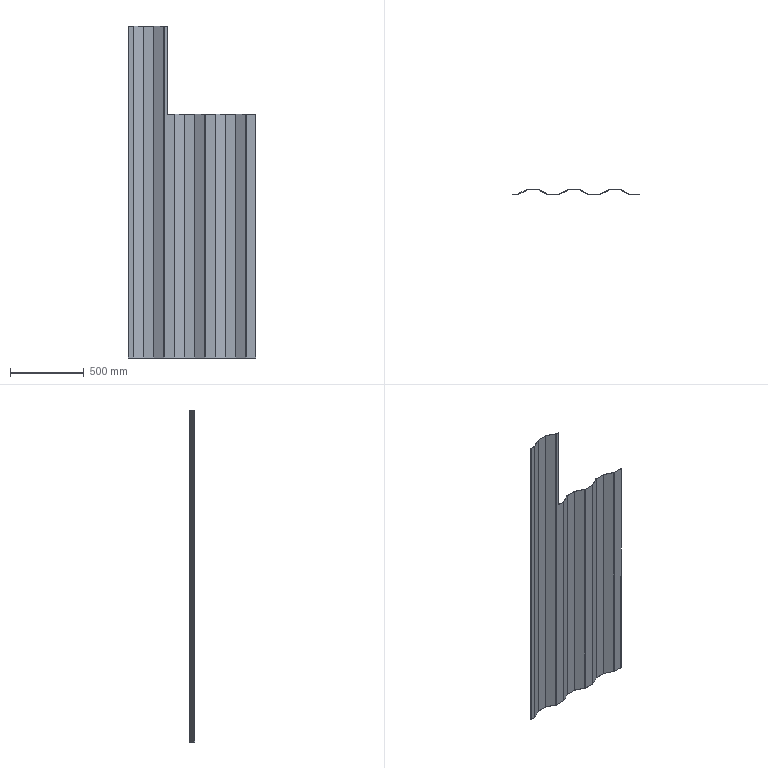Part | STEP file | 750038173 | 1 solid | 56 faces | box 865 x 36 x 2253 mm | volume 3353740 mm3 | plane 32 | cylinder 24 | commonest cylinder face diameters 6 x12 10 x12